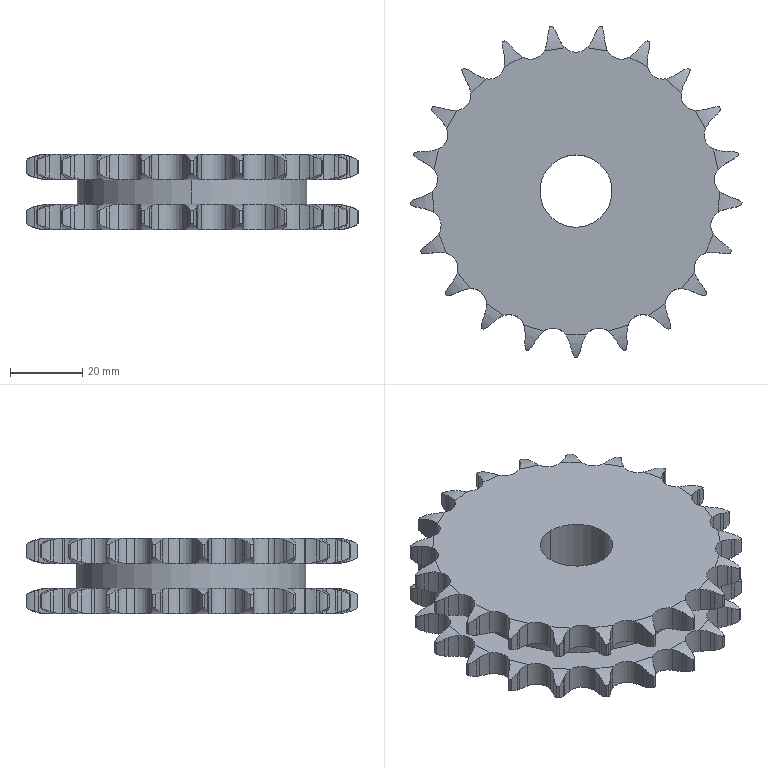Part | STEP file | 1 solid | 448 faces | box 91.67 x 91.415 x 20.973 mm | volume 88358 mm3 | cylinder 276 | plane 88 | spline 84 | commonest cylinder face diameters 14.045 x88 22.211 x88 8.595 x54 91.879 x42 20 x2 63.361 x2